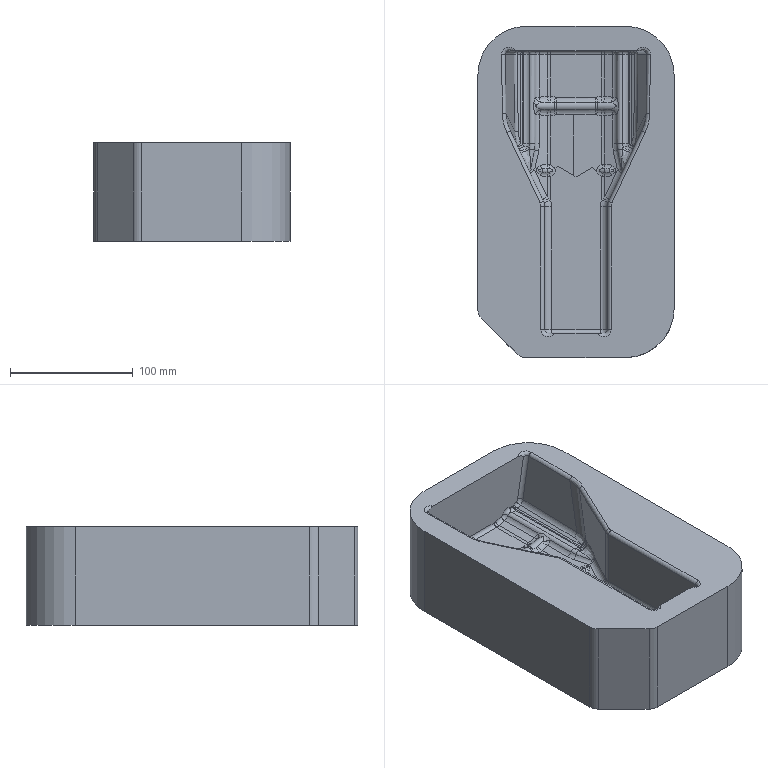NC program | NX | posted with a generic post | part box 160 x 270 x 80 mm
Lines 17065 to 17923 of 159324:
(ZLEVEL_CORNER , TOOL : D6)
N34122 M6
N34124 G54
N34126 G17 G0 G90 X-21.366 Y-109.488 S0 M3
N34128 G43 Z10. H0
N34130 Z-0.3
N34132 G94 G1 X-23.096 Y-109.678 F1500.
N34134 G3 X-19.596 Y-112.076 R3.
N34136 G2 X-19.061 Y-112.025 R2.979
N34138 G1 X-17.201
N34140 G3 X-14.201 Y-109.025 R3.
N34142 G0 X-21.093 Y-109.265 Z-0.45
N34144 G1 X-23.66 Y-109.832
N34146 G3 X-20.076 Y-112.102 R3.
N34148 G2 X-19.426 Y-112.025 R3.184
N34150 G1 X-17.104
N34152 G3 X-14.104 Y-109.025 R3.
N34154 G0 X-20.874 Y-109.14 Z-0.599
N34156 G1 X-22.229 Y-111.006
N34158 G3 X-20.418 Y-112.111 R1.5
N34160 G2 X-19.73 Y-112.025 R3.05
N34162 G1 X-16.975
N34164 G3 X-13.975 Y-109.025 R3.
N34166 G0 X-20.689 Y-109.066 Z-0.749
N34168 G1 X-22.622 Y-111.108
N34170 G3 X-20.764 Y-112.132 R1.5
N34172 G2 X-20. Y-112.025 R2.721
N34174 G1 X-16.859
N34176 G3 X-13.859 Y-109.025 R3.
N34178 G0 X-20.531 Y-109.033 Z-0.899
N34180 G1 X-22.984 Y-111.164
N34182 G3 X-21.11 Y-112.159 R1.5
N34184 G2 X-20.244 Y-112.025 R3.052
N34186 G1 X-16.754
N34188 G3 X-13.754 Y-109.025 R3.
N34190 G0 X-20.394 Z-1.049
N34192 G1 X-23.332 Y-111.249
N34194 G3 X-21.429 Y-112.188 R1.5
N34196 G2 X-20.47 Y-112.025 R3.073
N34198 G1 X-16.66
N34200 G3 X-13.66 Y-109.025 R3.
N34202 G0 X-20.274 Z-1.199
N34204 G1 X-22.854 Y-112.166
N34206 G3 X-21.707 Y-112.208 R1.5
N34208 G2 X-20.68 Y-112.025 R2.92
N34210 G1 X-16.575
N34212 G3 X-13.575 Y-109.025 R3.
N34214 G0 X-20.168 Z-1.349
N34216 G1 X-23.127 Y-112.21
N34218 G3 X-21.979 Y-112.234 R1.5
N34220 G2 X-20.878 Y-112.025 R3.066
N34222 G1 X-16.498
N34224 G3 X-13.498 Y-109.025 R3.
N34226 G0 X-19.189 Z-1.499
N34228 G1 Y-109.243
N34230 G3 X-22.189 Y-112.243 R3.
N34232 G2 X-21.067 Y-112.025 R3.084
N34234 G1 X-16.43
N34236 G3 X-13.43 Y-109.025 R3.
N34238 G0 X-19.434 Z-1.649
N34240 G1 Y-109.271
N34242 G3 X-22.434 Y-112.271 R3.
N34244 G2 X-21.246 Y-112.025 R2.934
N34246 G1 X-16.369
N34248 G3 X-13.369 Y-109.025 R3.
N34250 G0 X-19.734 Y-102.289 Z-2.398
N34252 G3 X-22.734 Y-105.289 R3.
N34254 G1 Y-112.025
N34256 Y-112.062
N34258 X-22.705 Y-112.088
N34260 X-22.668 Y-112.086
N34262 G2 X-22.065 Y-112.025 R3.236
N34264 G1 X-16.169
N34266 G3 X-13.169 Y-109.025 R3.
N34268 G0 X-19.707 Y-102.382 Z-2.548
N34270 G3 X-22.707 Y-105.382 R3.
N34272 G1 Y-112.025
N34274 X-22.709 Y-112.05
N34276 X-22.685 Y-112.057
N34278 G2 X-22.218 Y-112.025 R6.699
N34280 G1 X-16.148
N34282 G3 X-13.148 Y-109.025 R3.
N34284 G0 X-19.688 Y-102.435 Z-2.698
N34286 G3 X-22.688 Y-105.435 R3.
N34288 G1 Y-112.038
N34290 X-22.668 Y-112.04
N34292 X-22.37 Y-112.025
N34294 X-16.133
N34296 G3 X-13.133 Y-109.025 R3.
N34298 G0 X-19.677 Y-102.463 Z-2.847
N34300 G3 X-22.677 Y-105.463 R3.
N34302 G1 Y-112.029
N34304 X-22.55 Y-112.027
N34306 X-22.52 Y-112.025
N34308 X-16.124
N34310 G3 X-13.124 Y-109.025 R3.
N34312 G0 X-19.673 Y-102.475 Z-2.997
N34314 G3 X-22.673 Y-105.475 R3.
N34316 G1 Y-111.999
N34318 Y-112.026
N34320 X-22.668 Y-112.025
N34322 X-16.121
N34324 G3 X-13.121 Y-109.025 R3.
N34326 G0 X-19.673 Y-102.473 Z-3.147
N34328 G3 X-22.673 Y-105.473 R3.
N34330 G1 Y-112.025
N34332 X-16.121
N34334 G3 X-13.121 Y-109.025 R3.
N34336 G0 X-19.673 Y-102.473 Z-3.297
N34338 G3 X-22.673 Y-105.473 R3.
N34340 G1 Y-112.025
N34342 X-16.121
N34344 G3 X-13.121 Y-109.025 R3.
N34346 G0 X-19.673 Y-102.473 Z-3.447
N34348 G3 X-22.673 Y-105.473 R3.
N34350 G1 Y-112.025
N34352 X-16.121
N34354 G3 X-13.121 Y-109.025 R3.
N34356 G0 X-19.673 Y-102.473 Z-3.597
N34358 G3 X-22.673 Y-105.473 R3.
N34360 G1 Y-112.025
N34362 X-16.121
N34364 G3 X-13.121 Y-109.025 R3.
N34366 G0 X-19.673 Y-102.473 Z-3.747
N34368 G3 X-22.673 Y-105.473 R3.
N34370 G1 Y-112.025
N34372 X-16.121
N34374 G3 X-13.121 Y-109.025 R3.
N34376 G0 X-19.673 Y-102.473 Z-3.896
N34378 G3 X-22.673 Y-105.473 R3.
N34380 G1 Y-112.025
N34382 X-16.121
N34384 G3 X-13.121 Y-109.025 R3.
N34386 G0 X-19.673 Y-102.473 Z-4.046
N34388 G3 X-22.673 Y-105.473 R3.
N34390 G1 Y-112.025
N34392 X-16.121
N34394 G3 X-13.121 Y-109.025 R3.
N34396 G0 X-19.673 Y-102.473 Z-4.196
N34398 G3 X-22.673 Y-105.473 R3.
N34400 G1 Y-112.025
N34402 X-16.121
N34404 G3 X-13.121 Y-109.025 R3.
N34406 G0 X-19.673 Y-102.473 Z-4.346
N34408 G3 X-22.673 Y-105.473 R3.
N34410 G1 Y-112.025
N34412 X-16.121
N34414 G3 X-13.121 Y-109.025 R3.
N34416 G0 X-19.673 Y-102.473 Z-4.496
N34418 G3 X-22.673 Y-105.473 R3.
N34420 G1 Y-112.025
N34422 X-16.121
N34424 G3 X-13.121 Y-109.025 R3.
N34426 G0 X-19.673 Y-102.473 Z-4.646
N34428 G3 X-22.673 Y-105.473 R3.
N34430 G1 Y-112.025
N34432 X-16.121
N34434 G3 X-13.121 Y-109.025 R3.
N34436 G0 X-19.673 Y-102.473 Z-4.796
N34438 G3 X-22.673 Y-105.473 R3.
N34440 G1 Y-112.025
N34442 X-16.121
N34444 G3 X-13.121 Y-109.025 R3.
N34446 G0 X-19.673 Y-102.473 Z-4.946
N34448 G3 X-22.673 Y-105.473 R3.
N34450 G1 Y-112.025
N34452 X-16.121
N34454 G3 X-13.121 Y-109.025 R3.
N34456 G0 X-19.673 Y-102.473 Z-5.095
N34458 G3 X-22.673 Y-105.473 R3.
N34460 G1 Y-112.025
N34462 X-16.121
N34464 G3 X-13.121 Y-109.025 R3.
N34466 G0 X-19.673 Y-102.473 Z-5.245
N34468 G3 X-22.673 Y-105.473 R3.
N34470 G1 Y-112.025
N34472 X-16.121
N34474 G3 X-13.121 Y-109.025 R3.
N34476 G0 X-19.673 Y-102.473 Z-5.395
N34478 G3 X-22.673 Y-105.473 R3.
N34480 G1 Y-112.025
N34482 X-16.121
N34484 G3 X-13.121 Y-109.025 R3.
N34486 G0 X-19.673 Y-102.473 Z-5.545
N34488 G3 X-22.673 Y-105.473 R3.
N34490 G1 Y-112.025
N34492 X-16.121
N34494 G3 X-13.121 Y-109.025 R3.
N34496 G0 X-19.673 Y-102.473 Z-5.695
N34498 G3 X-22.673 Y-105.473 R3.
N34500 G1 Y-112.025
N34502 X-16.121
N34504 G3 X-13.121 Y-109.025 R3.
N34506 G0 X-19.673 Y-102.473 Z-5.845
N34508 G3 X-22.673 Y-105.473 R3.
N34510 G1 Y-112.025
N34512 X-16.121
N34514 G3 X-13.121 Y-109.025 R3.
N34516 G0 X-19.673 Y-102.473 Z-5.995
N34518 G3 X-22.673 Y-105.473 R3.
N34520 G1 Y-112.025
N34522 X-16.121
N34524 G3 X-13.121 Y-109.025 R3.
N34526 G0 X-19.673 Y-102.473 Z-6.144
N34528 G3 X-22.673 Y-105.473 R3.
N34530 G1 Y-112.025
N34532 X-16.121
N34534 G3 X-13.121 Y-109.025 R3.
N34536 G0 X-19.673 Y-102.473 Z-6.294
N34538 G3 X-22.673 Y-105.473 R3.
N34540 G1 Y-112.025
N34542 X-16.121
N34544 G3 X-13.121 Y-109.025 R3.
N34546 G0 X-19.673 Y-102.473 Z-6.444
N34548 G3 X-22.673 Y-105.473 R3.
N34550 G1 Y-112.025
N34552 X-16.121
N34554 G3 X-13.121 Y-109.025 R3.
N34556 G0 X-19.673 Y-102.473 Z-6.594
N34558 G3 X-22.673 Y-105.473 R3.
N34560 G1 Y-112.025
N34562 X-16.121
N34564 G3 X-13.121 Y-109.025 R3.
N34566 G0 X-19.673 Y-102.473 Z-6.744
N34568 G3 X-22.673 Y-105.473 R3.
N34570 G1 Y-112.025
N34572 X-16.121
N34574 G3 X-13.121 Y-109.025 R3.
N34576 G0 X-19.673 Y-102.473 Z-6.894
N34578 G3 X-22.673 Y-105.473 R3.
N34580 G1 Y-112.025
N34582 X-16.121
N34584 G3 X-13.121 Y-109.025 R3.
N34586 G0 X-19.673 Y-102.473 Z-7.044
N34588 G3 X-22.673 Y-105.473 R3.
N34590 G1 Y-112.025
N34592 X-16.121
N34594 G3 X-13.121 Y-109.025 R3.
N34596 G0 X-19.673 Y-102.473 Z-7.193
N34598 G3 X-22.673 Y-105.473 R3.
N34600 G1 Y-112.025
N34602 X-16.121
N34604 G3 X-13.121 Y-109.025 R3.
N34606 G0 X-19.673 Y-102.473 Z-7.343
N34608 G3 X-22.673 Y-105.473 R3.
N34610 G1 Y-112.025
N34612 X-16.121
N34614 G3 X-13.121 Y-109.025 R3.
N34616 G0 X-19.673 Y-102.473 Z-7.493
N34618 G3 X-22.673 Y-105.473 R3.
N34620 G1 Y-112.025
N34622 X-16.121
N34624 G3 X-13.121 Y-109.025 R3.
N34626 G0 X-19.673 Y-102.473 Z-7.643
N34628 G3 X-22.673 Y-105.473 R3.
N34630 G1 Y-112.025
N34632 X-16.121
N34634 G3 X-13.121 Y-109.025 R3.
N34636 G0 X-19.673 Y-102.473 Z-7.793
N34638 G3 X-22.673 Y-105.473 R3.
N34640 G1 Y-112.025
N34642 X-16.121
N34644 G3 X-13.121 Y-109.025 R3.
N34646 G0 X-19.673 Y-102.473 Z-7.943
N34648 G3 X-22.673 Y-105.473 R3.
N34650 G1 Y-112.025
N34652 X-16.121
N34654 G3 X-13.121 Y-109.025 R3.
N34656 G0 X-19.673 Y-102.473 Z-8.093
N34658 G3 X-22.673 Y-105.473 R3.
N34660 G1 Y-112.025
N34662 X-16.121
N34664 G3 X-13.121 Y-109.025 R3.
N34666 G0 X-19.673 Y-102.473 Z-8.243
N34668 G3 X-22.673 Y-105.473 R3.
N34670 G1 Y-112.025
N34672 X-16.121
N34674 G3 X-13.121 Y-109.025 R3.
N34676 G0 X-19.673 Y-102.473 Z-8.392
N34678 G3 X-22.673 Y-105.473 R3.
N34680 G1 Y-112.025
N34682 X-16.121
N34684 G3 X-13.121 Y-109.025 R3.
N34686 G0 X-19.673 Y-102.473 Z-8.542
N34688 G3 X-22.673 Y-105.473 R3.
N34690 G1 Y-112.025
N34692 X-16.121
N34694 G3 X-13.121 Y-109.025 R3.
N34696 G0 X-19.673 Y-102.473 Z-8.692
N34698 G3 X-22.673 Y-105.473 R3.
N34700 G1 Y-112.025
N34702 X-16.121
N34704 G3 X-13.121 Y-109.025 R3.
N34706 G0 X-19.673 Y-102.473 Z-8.842
N34708 G3 X-22.673 Y-105.473 R3.
N34710 G1 Y-112.025
N34712 X-16.121
N34714 G3 X-13.121 Y-109.025 R3.
N34716 G0 X-19.673 Y-102.473 Z-8.992
N34718 G3 X-22.673 Y-105.473 R3.
N34720 G1 Y-112.025
N34722 X-16.121
N34724 G3 X-13.121 Y-109.025 R3.
N34726 G0 X-19.673 Y-102.473 Z-9.142
N34728 G3 X-22.673 Y-105.473 R3.
N34730 G1 Y-112.025
N34732 X-16.121
N34734 G3 X-13.121 Y-109.025 R3.
N34736 G0 X-19.673 Y-102.473 Z-9.292
N34738 G3 X-22.673 Y-105.473 R3.
N34740 G1 Y-112.025
N34742 X-16.121
N34744 G3 X-13.121 Y-109.025 R3.
N34746 G0 X-19.673 Y-102.473 Z-9.441
N34748 G3 X-22.673 Y-105.473 R3.
N34750 G1 Y-112.025
N34752 X-16.121
N34754 G3 X-13.121 Y-109.025 R3.
N34756 G0 X-19.673 Y-102.473 Z-9.591
N34758 G3 X-22.673 Y-105.473 R3.
N34760 G1 Y-112.025
N34762 X-16.121
N34764 G3 X-13.121 Y-109.025 R3.
N34766 G0 X-19.673 Y-102.473 Z-9.741
N34768 G3 X-22.673 Y-105.473 R3.
N34770 G1 Y-112.025
N34772 X-16.121
N34774 G3 X-13.121 Y-109.025 R3.
N34776 G0 X-19.673 Y-102.473 Z-9.891
N34778 G3 X-22.673 Y-105.473 R3.
N34780 G1 Y-112.025
N34782 X-16.121
N34784 G3 X-13.121 Y-109.025 R3.
N34786 G0 X-19.673 Y-102.473 Z-10.041
N34788 G3 X-22.673 Y-105.473 R3.
N34790 G1 Y-112.025
N34792 X-16.121
N34794 G3 X-13.121 Y-109.025 R3.
N34796 G0 X-19.673 Y-102.473 Z-10.191
N34798 G3 X-22.673 Y-105.473 R3.
N34800 G1 Y-112.025
N34802 X-16.121
N34804 G3 X-13.121 Y-109.025 R3.
N34806 G0 X-19.673 Y-102.473 Z-10.341
N34808 G3 X-22.673 Y-105.473 R3.
N34810 G1 Y-112.025
N34812 X-16.121
N34814 G3 X-13.121 Y-109.025 R3.
N34816 G0 X-19.673 Y-102.473 Z-10.49
N34818 G3 X-22.673 Y-105.473 R3.
N34820 G1 Y-112.025
N34822 X-16.121
N34824 G3 X-13.121 Y-109.025 R3.
N34826 G0 X-19.673 Y-102.473 Z-10.64
N34828 G3 X-22.673 Y-105.473 R3.
N34830 G1 Y-112.025
N34832 X-16.121
N34834 G3 X-13.121 Y-109.025 R3.
N34836 G0 X-19.673 Y-102.473 Z-10.79
N34838 G3 X-22.673 Y-105.473 R3.
N34840 G1 Y-112.025
N34842 X-16.121
N34844 G3 X-13.121 Y-109.025 R3.
N34846 G0 X-19.673 Y-102.473 Z-10.94
N34848 G3 X-22.673 Y-105.473 R3.
N34850 G1 Y-112.025
N34852 X-16.121
N34854 G3 X-13.121 Y-109.025 R3.
N34856 G0 X-19.673 Y-102.473 Z-11.09
N34858 G3 X-22.673 Y-105.473 R3.
N34860 G1 Y-112.025
N34862 X-16.121
N34864 G3 X-13.121 Y-109.025 R3.
N34866 G0 X-19.673 Y-102.473 Z-11.24
N34868 G3 X-22.673 Y-105.473 R3.
N34870 G1 Y-112.025
N34872 X-16.121
N34874 G3 X-13.121 Y-109.025 R3.
N34876 G0 X-19.673 Y-102.473 Z-11.39
N34878 G3 X-22.673 Y-105.473 R3.
N34880 G1 Y-112.025
N34882 X-16.121
N34884 G3 X-13.121 Y-109.025 R3.
N34886 G0 X-19.673 Y-102.473 Z-11.54
N34888 G3 X-22.673 Y-105.473 R3.
N34890 G1 Y-112.025
N34892 X-16.121
N34894 G3 X-13.121 Y-109.025 R3.
N34896 G0 X-19.673 Y-102.473 Z-11.689
N34898 G3 X-22.673 Y-105.473 R3.
N34900 G1 Y-112.025
N34902 X-16.121
N34904 G3 X-13.121 Y-109.025 R3.
N34906 G0 X-19.673 Y-102.473 Z-11.839
N34908 G3 X-22.673 Y-105.473 R3.
N34910 G1 Y-112.025
N34912 X-16.121
N34914 G3 X-13.121 Y-109.025 R3.
N34916 G0 X-19.673 Y-102.473 Z-11.989
N34918 G3 X-22.673 Y-105.473 R3.
N34920 G1 Y-112.025
N34922 X-16.121
N34924 G3 X-13.121 Y-109.025 R3.
N34926 G0 X-19.673 Y-102.473 Z-12.139
N34928 G3 X-22.673 Y-105.473 R3.
N34930 G1 Y-112.025
N34932 X-16.121
N34934 G3 X-13.121 Y-109.025 R3.
N34936 G0 X-19.673 Y-102.473 Z-12.289
N34938 G3 X-22.673 Y-105.473 R3.
N34940 G1 Y-112.025
N34942 X-16.121
N34944 G3 X-13.121 Y-109.025 R3.
N34946 G0 X-19.673 Y-102.473 Z-12.439
N34948 G3 X-22.673 Y-105.473 R3.
N34950 G1 Y-112.025
N34952 X-16.121
N34954 G3 X-13.121 Y-109.025 R3.
N34956 G0 X-19.673 Y-102.473 Z-12.589
N34958 G3 X-22.673 Y-105.473 R3.
N34960 G1 Y-112.025
N34962 X-16.121
N34964 G3 X-13.121 Y-109.025 R3.
N34966 G0 X-19.673 Y-102.473 Z-12.738
N34968 G3 X-22.673 Y-105.473 R3.
N34970 G1 Y-112.025
N34972 X-16.121
N34974 G3 X-13.121 Y-109.025 R3.
N34976 G0 X-19.673 Y-102.473 Z-12.888
N34978 G3 X-22.673 Y-105.473 R3.
N34980 G1 Y-112.025
N34982 X-16.121
N34984 G3 X-13.121 Y-109.025 R3.
N34986 G0 X-19.673 Y-102.473 Z-13.038
N34988 G3 X-22.673 Y-105.473 R3.
N34990 G1 Y-112.025
N34992 X-16.121
N34994 G3 X-13.121 Y-109.025 R3.
N34996 G0 X-19.673 Y-102.473 Z-13.188
N34998 G3 X-22.673 Y-105.473 R3.
N35000 G1 Y-112.025
N35002 X-16.121
N35004 G3 X-13.121 Y-109.025 R3.
N35006 G0 X-19.673 Y-102.473 Z-13.338
N35008 G3 X-22.673 Y-105.473 R3.
N35010 G1 Y-112.025
N35012 X-16.121
N35014 G3 X-13.121 Y-109.025 R3.
N35016 G0 X-19.673 Y-102.473 Z-13.488
N35018 G3 X-22.673 Y-105.473 R3.
N35020 G1 Y-112.025
N35022 X-16.121
N35024 G3 X-13.121 Y-109.025 R3.
N35026 G0 X-19.673 Y-102.473 Z-13.638
N35028 G3 X-22.673 Y-105.473 R3.
N35030 G1 Y-112.025
N35032 X-16.121
N35034 G3 X-13.121 Y-109.025 R3.
N35036 G0 X-19.673 Y-102.473 Z-13.787
N35038 G3 X-22.673 Y-105.473 R3.
N35040 G1 Y-112.025
N35042 X-16.121
N35044 G3 X-13.121 Y-109.025 R3.
N35046 G0 X-19.673 Y-102.473 Z-13.937
N35048 G3 X-22.673 Y-105.473 R3.
N35050 G1 Y-112.025
N35052 X-16.121
N35054 G3 X-13.121 Y-109.025 R3.
N35056 G0 X-19.673 Y-102.473 Z-14.087
N35058 G3 X-22.673 Y-105.473 R3.
N35060 G1 Y-112.025
N35062 X-16.121
N35064 G3 X-13.121 Y-109.025 R3.
N35066 G0 X-19.673 Y-102.473 Z-14.237
N35068 G3 X-22.673 Y-105.473 R3.
N35070 G1 Y-112.025
N35072 X-16.121
N35074 G3 X-13.121 Y-109.025 R3.
N35076 G0 X-19.673 Y-102.473 Z-14.387
N35078 G3 X-22.673 Y-105.473 R3.
N35080 G1 Y-112.025
N35082 X-16.121
N35084 G3 X-13.121 Y-109.025 R3.
N35086 G0 X-19.673 Y-102.473 Z-14.537
N35088 G3 X-22.673 Y-105.473 R3.
N35090 G1 Y-112.025
N35092 X-16.121
N35094 G3 X-13.121 Y-109.025 R3.
N35096 G0 X-19.673 Y-102.473 Z-14.687
N35098 G3 X-22.673 Y-105.473 R3.
N35100 G1 Y-112.025
N35102 X-16.121
N35104 G3 X-13.121 Y-109.025 R3.
N35106 G0 X-19.673 Y-102.473 Z-14.837
N35108 G3 X-22.673 Y-105.473 R3.
N35110 G1 Y-112.025
N35112 X-16.121
N35114 G3 X-13.121 Y-109.025 R3.
N35116 G0 X-19.673 Y-102.473 Z-14.986
N35118 G3 X-22.673 Y-105.473 R3.
N35120 G1 Y-112.025
N35122 X-16.121
N35124 G3 X-13.121 Y-109.025 R3.
N35126 G0 X-19.673 Y-102.473 Z-15.136
N35128 G3 X-22.673 Y-105.473 R3.
N35130 G1 Y-112.025
N35132 X-16.121
N35134 G3 X-13.121 Y-109.025 R3.
N35136 G0 X-19.673 Y-102.473 Z-15.286
N35138 G3 X-22.673 Y-105.473 R3.
N35140 G1 Y-112.025
N35142 X-16.121
N35144 G3 X-13.121 Y-109.025 R3.
N35146 G0 X-19.673 Y-102.473 Z-15.436
N35148 G3 X-22.673 Y-105.473 R3.
N35150 G1 Y-112.025
N35152 X-16.121
N35154 G3 X-13.121 Y-109.025 R3.
N35156 G0 X-19.673 Y-102.473 Z-15.586
N35158 G3 X-22.673 Y-105.473 R3.
N35160 G1 Y-112.025
N35162 X-16.121
N35164 G3 X-13.121 Y-109.025 R3.
N35166 G0 X-19.673 Y-102.473 Z-15.736
N35168 G3 X-22.673 Y-105.473 R3.
N35170 G1 Y-112.025
N35172 X-16.121
N35174 G3 X-13.121 Y-109.025 R3.
N35176 G0 X-19.673 Y-102.473 Z-15.886
N35178 G3 X-22.673 Y-105.473 R3.
N35180 G1 Y-112.025
N35182 X-16.121
N35184 G3 X-13.121 Y-109.025 R3.
N35186 G0 X-19.673 Y-102.473 Z-16.035
N35188 G3 X-22.673 Y-105.473 R3.
N35190 G1 Y-112.025
N35192 X-16.121
N35194 G3 X-13.121 Y-109.025 R3.
N35196 G0 X-19.673 Y-102.473 Z-16.185
N35198 G3 X-22.673 Y-105.473 R3.
N35200 G1 Y-112.025
N35202 X-16.121
N35204 G3 X-13.121 Y-109.025 R3.
N35206 G0 X-19.673 Y-102.473 Z-16.335
N35208 G3 X-22.673 Y-105.473 R3.
N35210 G1 Y-112.025
N35212 X-16.121
N35214 G3 X-13.121 Y-109.025 R3.
N35216 G0 X-19.673 Y-102.473 Z-16.485
N35218 G3 X-22.673 Y-105.473 R3.
N35220 G1 Y-112.025
N35222 X-16.121
N35224 G3 X-13.121 Y-109.025 R3.
N35226 G0 X-19.673 Y-102.473 Z-16.635
N35228 G3 X-22.673 Y-105.473 R3.
N35230 G1 Y-112.025
N35232 X-16.121
N35234 G3 X-13.121 Y-109.025 R3.
N35236 G0 X-19.673 Y-102.473 Z-16.785
N35238 G3 X-22.673 Y-105.473 R3.
N35240 G1 Y-112.025
N35242 X-16.121
N35244 G3 X-13.121 Y-109.025 R3.
N35246 G0 X-19.673 Y-102.473 Z-16.935
N35248 G3 X-22.673 Y-105.473 R3.
N35250 G1 Y-112.025
N35252 X-16.121
N35254 G3 X-13.121 Y-109.025 R3.
N35256 G0 X-19.673 Y-102.473 Z-17.084
N35258 G3 X-22.673 Y-105.473 R3.
N35260 G1 Y-112.025
N35262 X-16.121
N35264 G3 X-13.121 Y-109.025 R3.
N35266 G0 X-19.673 Y-102.473 Z-17.234
N35268 G3 X-22.673 Y-105.473 R3.
N35270 G1 Y-112.025
N35272 X-16.121
N35274 G3 X-13.121 Y-109.025 R3.
N35276 G0 X-19.673 Y-102.473 Z-17.384
N35278 G3 X-22.673 Y-105.473 R3.
N35280 G1 Y-112.025
N35282 X-16.121
N35284 G3 X-13.121 Y-109.025 R3.
N35286 G0 X-19.673 Y-102.473 Z-17.534
N35288 G3 X-22.673 Y-105.473 R3.
N35290 G1 Y-112.025
N35292 X-16.121
N35294 G3 X-13.121 Y-109.025 R3.
N35296 G0 X-19.673 Y-102.473 Z-17.684
N35298 G3 X-22.673 Y-105.473 R3.
N35300 G1 Y-112.025
N35302 X-16.121
N35304 G3 X-13.121 Y-109.025 R3.
N35306 G0 X-19.673 Y-102.473 Z-17.834
N35308 G3 X-22.673 Y-105.473 R3.
N35310 G1 Y-112.025
N35312 X-16.121
N35314 G3 X-13.121 Y-109.025 R3.
N35316 G0 X-19.673 Y-102.473 Z-17.984
N35318 G3 X-22.673 Y-105.473 R3.
N35320 G1 Y-112.025
N35322 X-16.121
N35324 G3 X-13.121 Y-109.025 R3.
N35326 G0 X-19.673 Y-102.473 Z-18.134
N35328 G3 X-22.673 Y-105.473 R3.
N35330 G1 Y-112.025
N35332 X-16.121
N35334 G3 X-13.121 Y-109.025 R3.
N35336 G0 X-19.673 Y-102.473 Z-18.283
N35338 G3 X-22.673 Y-105.473 R3.
N35340 G1 Y-112.025
N35342 X-16.121
N35344 G3 X-13.121 Y-109.025 R3.
N35346 G0 X-19.673 Y-102.473 Z-18.433
N35348 G3 X-22.673 Y-105.473 R3.
N35350 G1 Y-112.025
N35352 X-16.121
N35354 G3 X-13.121 Y-109.025 R3.
N35356 G0 X-19.673 Y-102.473 Z-18.583
N35358 G3 X-22.673 Y-105.473 R3.
N35360 G1 Y-112.025
N35362 X-16.121
N35364 G3 X-13.121 Y-109.025 R3.
N35366 G0 X-19.673 Y-102.473 Z-18.733
N35368 G3 X-22.673 Y-105.473 R3.
N35370 G1 Y-112.025
N35372 X-16.121
N35374 G3 X-13.121 Y-109.025 R3.
N35376 G0 X-19.673 Y-102.473 Z-18.883
N35378 G3 X-22.673 Y-105.473 R3.
N35380 G1 Y-112.025
N35382 X-16.121
N35384 G3 X-13.121 Y-109.025 R3.
N35386 G0 X-19.673 Y-102.473 Z-19.033
N35388 G3 X-22.673 Y-105.473 R3.
N35390 G1 Y-112.025
N35392 X-16.121
N35394 G3 X-13.121 Y-109.025 R3.
N35396 G0 X-19.673 Y-102.473 Z-19.183
N35398 G3 X-22.673 Y-105.473 R3.
N35400 G1 Y-112.025
N35402 X-16.121
N35404 G3 X-13.121 Y-109.025 R3.
N35406 G0 X-19.673 Y-102.473 Z-19.332
N35408 G3 X-22.673 Y-105.473 R3.
N35410 G1 Y-112.025
N35412 X-16.121
N35414 G3 X-13.121 Y-109.025 R3.
N35416 G0 X-19.673 Y-102.473 Z-19.482
N35418 G3 X-22.673 Y-105.473 R3.
N35420 G1 Y-112.025
N35422 X-16.121
N35424 G3 X-13.121 Y-109.025 R3.
N35426 G0 X-19.673 Y-102.473 Z-19.632
N35428 G3 X-22.673 Y-105.473 R3.
N35430 G1 Y-112.025
N35432 X-16.121
N35434 G3 X-13.121 Y-109.025 R3.
N35436 G0 X-19.673 Y-102.473 Z-19.782
N35438 G3 X-22.673 Y-105.473 R3.
N35440 G1 Y-112.025
N35442 X-16.121
N35444 G3 X-13.121 Y-109.025 R3.
N35446 G0 X-19.673 Y-102.473 Z-19.932
N35448 G3 X-22.673 Y-105.473 R3.
N35450 G1 Y-112.025
N35452 X-16.121
N35454 G3 X-13.121 Y-109.025 R3.
N35456 G0 X-19.673 Y-102.473 Z-20.082
N35458 G3 X-22.673 Y-105.473 R3.
N35460 G1 Y-112.025
N35462 X-16.121
N35464 G3 X-13.121 Y-109.025 R3.
N35466 G0 X-19.673 Y-102.473 Z-20.232
N35468 G3 X-22.673 Y-105.473 R3.
N35470 G1 Y-112.025
N35472 X-16.121
N35474 G3 X-13.121 Y-109.025 R3.
N35476 G0 X-19.673 Y-102.473 Z-20.381
N35478 G3 X-22.673 Y-105.473 R3.
N35480 G1 Y-112.025
N35482 X-16.121
N35484 G3 X-13.121 Y-109.025 R3.
N35486 G0 X-19.673 Y-102.473 Z-20.531
N35488 G3 X-22.673 Y-105.473 R3.
N35490 G1 Y-112.025
N35492 X-16.121
N35494 G3 X-13.121 Y-109.025 R3.
N35496 G0 X-19.673 Y-102.473 Z-20.681
N35498 G3 X-22.673 Y-105.473 R3.
N35500 G1 Y-112.025
N35502 X-16.121
N35504 G3 X-13.121 Y-109.025 R3.
N35506 G0 X-19.673 Y-102.473 Z-20.831
N35508 G3 X-22.673 Y-105.473 R3.
N35510 G1 Y-112.025
N35512 X-16.121
N35514 G3 X-13.121 Y-109.025 R3.
N35516 G0 X-19.673 Y-102.473 Z-20.981
N35518 G3 X-22.673 Y-105.473 R3.
N35520 G1 Y-112.025
N35522 X-16.121
N35524 G3 X-13.121 Y-109.025 R3.
N35526 G0 X-19.673 Y-102.473 Z-21.131
N35528 G3 X-22.673 Y-105.473 R3.
N35530 G1 Y-112.025
N35532 X-16.121
N35534 G3 X-13.121 Y-109.025 R3.
N35536 G0 X-19.673 Y-102.473 Z-21.281
N35538 G3 X-22.673 Y-105.473 R3.
N35540 G1 Y-112.025
N35542 X-16.121
N35544 G3 X-13.121 Y-109.025 R3.
N35546 G0 X-19.673 Y-102.473 Z-21.431
N35548 G3 X-22.673 Y-105.473 R3.
N35550 G1 Y-112.025
N35552 X-16.121
N35554 G3 X-13.121 Y-109.025 R3.
N35556 G0 X-19.673 Y-102.473 Z-21.58
N35558 G3 X-22.673 Y-105.473 R3.
N35560 G1 Y-112.025
N35562 X-16.121
N35564 G3 X-13.121 Y-109.025 R3.
N35566 G0 X-19.673 Y-102.473 Z-21.73
N35568 G3 X-22.673 Y-105.473 R3.
N35570 G1 Y-112.025
N35572 X-16.121
N35574 G3 X-13.121 Y-109.025 R3.
N35576 G0 X-19.673 Y-102.473 Z-21.88
N35578 G3 X-22.673 Y-105.473 R3.
N35580 G1 Y-112.025
N35582 X-16.121
N35584 G3 X-13.121 Y-109.025 R3.
N35586 G0 X-19.673 Y-102.473 Z-22.03
N35588 G3 X-22.673 Y-105.473 R3.
N35590 G1 Y-112.025
N35592 X-16.121
N35594 G3 X-13.121 Y-109.025 R3.
N35596 G0 X-19.673 Y-102.473 Z-22.18
N35598 G3 X-22.673 Y-105.473 R3.
N35600 G1 Y-112.025
N35602 X-16.121
N35604 G3 X-13.121 Y-109.025 R3.
N35606 G0 X-19.673 Y-102.473 Z-22.33
N35608 G3 X-22.673 Y-105.473 R3.
N35610 G1 Y-112.025
N35612 X-16.121
N35614 G3 X-13.121 Y-109.025 R3.
N35616 G0 X-19.673 Y-102.473 Z-22.48
N35618 G3 X-22.673 Y-105.473 R3.
N35620 G1 Y-112.025
N35622 X-16.121
N35624 G3 X-13.121 Y-109.025 R3.
N35626 G0 X-19.673 Y-102.473 Z-22.629
N35628 G3 X-22.673 Y-105.473 R3.
N35630 G1 Y-112.025
N35632 X-16.121
N35634 G3 X-13.121 Y-109.025 R3.
N35636 G0 X-19.673 Y-102.473 Z-22.779
N35638 G3 X-22.673 Y-105.473 R3.
N35640 G1 Y-112.025
N35642 X-16.121
N35644 G3 X-13.121 Y-109.025 R3.
N35646 G0 X-19.673 Y-102.473 Z-22.929
N35648 G3 X-22.673 Y-105.473 R3.
N35650 G1 Y-112.025
N35652 X-16.121
N35654 G3 X-13.121 Y-109.025 R3.
N35656 G0 X-19.673 Y-102.473 Z-23.079
N35658 G3 X-22.673 Y-105.473 R3.
N35660 G1 Y-112.025
N35662 X-16.121
N35664 G3 X-13.121 Y-109.025 R3.
N35666 G0 X-19.673 Y-102.473 Z-23.229
N35668 G3 X-22.673 Y-105.473 R3.
N35670 G1 Y-112.025
N35672 X-16.121
N35674 G3 X-13.121 Y-109.025 R3.
N35676 G0 X-19.673 Y-102.473 Z-23.379
N35678 G3 X-22.673 Y-105.473 R3.
N35680 G1 Y-112.025
N35682 X-16.121
N35684 G3 X-13.121 Y-109.025 R3.
N35686 G0 X-19.673 Y-102.473 Z-23.529
N35688 G3 X-22.673 Y-105.473 R3.
N35690 G1 Y-112.025
N35692 X-16.121
N35694 G3 X-13.121 Y-109.025 R3.
N35696 G0 X-19.673 Y-102.473 Z-23.678
N35698 G3 X-22.673 Y-105.473 R3.
N35700 G1 Y-112.025
N35702 X-16.121
N35704 G3 X-13.121 Y-109.025 R3.
N35706 G0 X-19.673 Y-102.473 Z-23.828
N35708 G3 X-22.673 Y-105.473 R3.
N35710 G1 Y-112.025
N35712 X-16.121
N35714 G3 X-13.121 Y-109.025 R3.
N35716 G0 X-19.673 Y-102.473 Z-23.978
N35718 G3 X-22.673 Y-105.473 R3.
N35720 G1 Y-112.025
N35722 X-16.121
N35724 G3 X-13.121 Y-109.025 R3.
N35726 G0 X-19.673 Y-102.473 Z-24.128
N35728 G3 X-22.673 Y-105.473 R3.
N35730 G1 Y-112.025
N35732 X-16.121
N35734 G3 X-13.121 Y-109.025 R3.
N35736 G0 X-19.673 Y-102.473 Z-24.278
N35738 G3 X-22.673 Y-105.473 R3.
N35740 G1 Y-112.025
N35742 X-16.121
N35744 G3 X-13.121 Y-109.025 R3.
N35746 G0 X-19.673 Y-102.473 Z-24.428
N35748 G3 X-22.673 Y-105.473 R3.
N35750 G1 Y-112.025
N35752 X-16.121
N35754 G3 X-13.121 Y-109.025 R3.
N35756 G0 X-19.673 Y-102.473 Z-24.578
N35758 G3 X-22.673 Y-105.473 R3.
N35760 G1 Y-112.025
N35762 X-16.121
N35764 G3 X-13.121 Y-109.025 R3.
N35766 G0 X-19.673 Y-102.473 Z-24.728
N35768 G3 X-22.673 Y-105.473 R3.
N35770 G1 Y-112.025
N35772 X-16.121
N35774 G3 X-13.121 Y-109.025 R3.
N35776 G0 X-19.673 Y-102.473 Z-24.877
N35778 G3 X-22.673 Y-105.473 R3.
N35780 G1 Y-112.025
N35782 X-16.121
N35784 G3 X-13.121 Y-109.025 R3.
N35786 G0 X-19.673 Y-102.473 Z-25.027
N35788 G3 X-22.673 Y-105.473 R3.
N35790 G1 Y-112.025
N35792 X-16.121
N35794 G3 X-13.121 Y-109.025 R3.
N35796 G0 X-19.673 Y-102.473 Z-25.177
N35798 G3 X-22.673 Y-105.473 R3.
N35800 G1 Y-112.025
N35802 X-16.121
N35804 G3 X-13.121 Y-109.025 R3.
N35806 G0 X-19.673 Y-102.473 Z-25.327
N35808 G3 X-22.673 Y-105.473 R3.
N35810 G1 Y-112.025
N35812 X-16.121
N35814 G3 X-13.121 Y-109.025 R3.
N35816 G0 X-19.673 Y-102.473 Z-25.477
N35818 G3 X-22.673 Y-105.473 R3.
N35820 G1 Y-112.025
N35822 X-16.121
N35824 G3 X-13.121 Y-109.025 R3.
N35826 G0 X-19.673 Y-102.473 Z-25.627
N35828 G3 X-22.673 Y-105.473 R3.
N35830 G1 Y-112.025
N35832 X-16.121